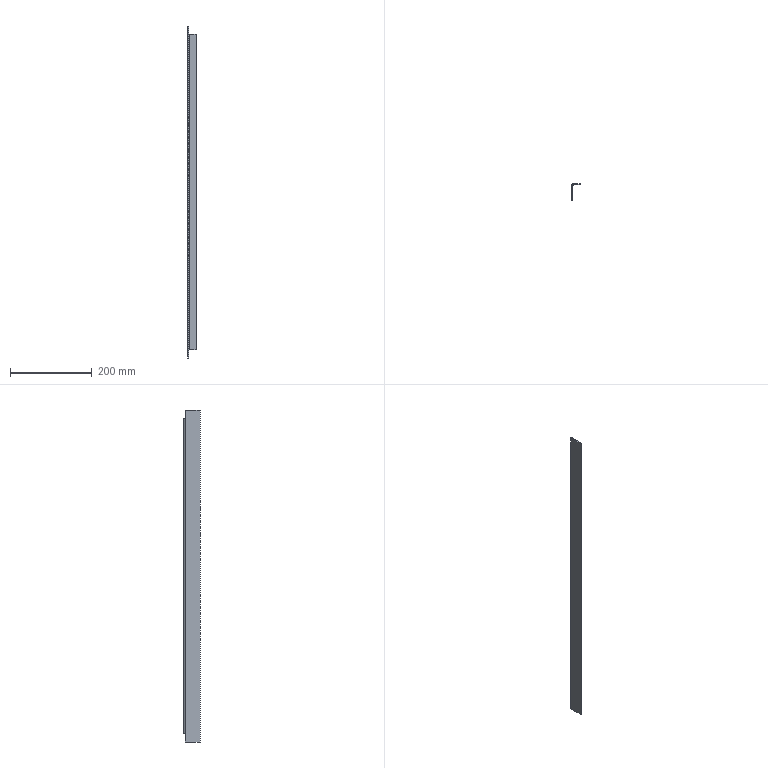Part | SolidWorks | features SMBaseFlange 2, FlatPattern 1, SheetMetal 1 | 1 solid | 16 faces | box 20 x 40 x 810 mm | volume 90217 mm3 | plane 14 | cylinder 2 | commonest cylinder face diameters 4 x1 8 x1
STEP:
#1=CARTESIAN_POINT('',(4.,40.,770.));
#2=VERTEX_POINT('',#1);
#3=CARTESIAN_POINT('',(4.,38.,770.));
#4=VERTEX_POINT('',#3);
#5=CARTESIAN_POINT('',(4.,40.,770.));
#6=DIRECTION('',(0.,-1.,0.));
#7=VECTOR('',#6,1000.);
#8=LINE('',#5,#7);
#9=EDGE_CURVE('',#2,#4,#8,.T.);
#10=ORIENTED_EDGE('',*,*,#9,.F.);
#11=CARTESIAN_POINT('',(0.,36.,770.));
#12=VERTEX_POINT('',#11);
#13=CARTESIAN_POINT('',(4.,36.,770.));
#14=DIRECTION('',(0.,0.,-1.));
#15=DIRECTION('',(1.,0.,0.));
#16=AXIS2_PLACEMENT_3D('',#13,#14,#15);
#17=CIRCLE('',#16,4.);
#18=EDGE_CURVE('',#12,#2,#17,.T.);
#19=ORIENTED_EDGE('',*,*,#18,.F.);
#20=CARTESIAN_POINT('',(2.,36.,770.));
#21=VERTEX_POINT('',#20);
#22=CARTESIAN_POINT('',(2.,36.,770.));
#23=DIRECTION('',(-1.,0.,0.));
#24=VECTOR('',#23,1000.);
#25=LINE('',#22,#24);
#26=EDGE_CURVE('',#21,#12,#25,.T.);
#27=ORIENTED_EDGE('',*,*,#26,.F.);
#28=CARTESIAN_POINT('',(4.,36.,770.));
#29=DIRECTION('',(0.,0.,-1.));
#30=DIRECTION('',(1.,0.,0.));
#31=AXIS2_PLACEMENT_3D('',#28,#29,#30);
#32=CIRCLE('',#31,2.);
#33=EDGE_CURVE('',#21,#4,#32,.T.);
#34=ORIENTED_EDGE('',*,*,#33,.T.);
#35=EDGE_LOOP('',(#10,#19,#27,#34));
#36=FACE_OUTER_BOUND('',#35,.T.);
#37=CARTESIAN_POINT('',(4.,40.,770.));
#38=DIRECTION('',(0.,0.,1.));
#39=DIRECTION('',(1.,0.,0.));
#40=AXIS2_PLACEMENT_3D('',#37,#38,#39);
#41=PLANE('',#40);
#42=ADVANCED_FACE('',(#36),#41,.T.);
#43=CARTESIAN_POINT('',(20.,40.,770.));
#44=VERTEX_POINT('',#43);
#45=CARTESIAN_POINT('',(0.,40.,770.));
#46=DIRECTION('',(1.,0.,0.));
#47=VECTOR('',#46,1000.);
#48=LINE('',#45,#47);
#49=EDGE_CURVE('',#2,#44,#48,.T.);
#50=ORIENTED_EDGE('',*,*,#49,.F.);
#51=ORIENTED_EDGE('',*,*,#9,.T.);
#52=CARTESIAN_POINT('',(20.,38.,770.));
#53=VERTEX_POINT('',#52);
#54=CARTESIAN_POINT('',(0.,38.,770.));
#55=DIRECTION('',(1.,0.,0.));
#56=VECTOR('',#55,1000.);
#57=LINE('',#54,#56);
#58=EDGE_CURVE('',#4,#53,#57,.T.);
#59=ORIENTED_EDGE('',*,*,#58,.T.);
#60=CARTESIAN_POINT('',(20.,40.,770.));
#61=DIRECTION('',(0.,-1.,0.));
#62=VECTOR('',#61,1000.);
#63=LINE('',#60,#62);
#64=EDGE_CURVE('',#44,#53,#63,.T.);
#65=ORIENTED_EDGE('',*,*,#64,.F.);
#66=EDGE_LOOP('',(#50,#51,#59,#65));
#67=FACE_OUTER_BOUND('',#66,.T.);
#68=CARTESIAN_POINT('',(2.,36.,770.));
#69=DIRECTION('',(0.,0.,1.));
#70=DIRECTION('',(1.,0.,0.));
#71=AXIS2_PLACEMENT_3D('',#68,#69,#70);
#72=PLANE('',#71);
#73=ADVANCED_FACE('',(#67),#72,.T.);
#74=CARTESIAN_POINT('',(0.,36.,0.));
#75=VERTEX_POINT('',#74);
#76=CARTESIAN_POINT('',(2.,36.,0.));
#77=VERTEX_POINT('',#76);
#78=CARTESIAN_POINT('',(0.,36.,0.));
#79=DIRECTION('',(1.,0.,0.));
#80=VECTOR('',#79,1000.);
#81=LINE('',#78,#80);
#82=EDGE_CURVE('',#75,#77,#81,.T.);
#83=ORIENTED_EDGE('',*,*,#82,.F.);
#84=CARTESIAN_POINT('',(4.,40.,0.));
#85=VERTEX_POINT('',#84);
#86=CARTESIAN_POINT('',(4.,36.,0.));
#87=DIRECTION('',(0.,0.,-1.));
#88=DIRECTION('',(1.,0.,0.));
#89=AXIS2_PLACEMENT_3D('',#86,#87,#88);
#90=CIRCLE('',#89,4.);
#91=EDGE_CURVE('',#75,#85,#90,.T.);
#92=ORIENTED_EDGE('',*,*,#91,.T.);
#93=CARTESIAN_POINT('',(4.,38.,0.));
#94=VERTEX_POINT('',#93);
#95=CARTESIAN_POINT('',(4.,38.,0.));
#96=DIRECTION('',(0.,1.,0.));
#97=VECTOR('',#96,1000.);
#98=LINE('',#95,#97);
#99=EDGE_CURVE('',#94,#85,#98,.T.);
#100=ORIENTED_EDGE('',*,*,#99,.F.);
#101=CARTESIAN_POINT('',(4.,36.,0.));
#102=DIRECTION('',(0.,0.,-1.));
#103=DIRECTION('',(1.,0.,0.));
#104=AXIS2_PLACEMENT_3D('',#101,#102,#103);
#105=CIRCLE('',#104,2.);
#106=EDGE_CURVE('',#77,#94,#105,.T.);
#107=ORIENTED_EDGE('',*,*,#106,.F.);
#108=EDGE_LOOP('',(#83,#92,#100,#107));
#109=FACE_OUTER_BOUND('',#108,.T.);
#110=CARTESIAN_POINT('',(0.,36.,0.));
#111=DIRECTION('',(0.,0.,-1.));
#112=DIRECTION('',(-1.,0.,0.));
#113=AXIS2_PLACEMENT_3D('',#110,#111,#112);
#114=PLANE('',#113);
#115=ADVANCED_FACE('',(#109),#114,.T.);
#116=CARTESIAN_POINT('',(20.,38.,0.));
#117=VERTEX_POINT('',#116);
#118=CARTESIAN_POINT('',(0.,38.,0.));
#119=DIRECTION('',(1.,0.,0.));
#120=VECTOR('',#119,1000.);
#121=LINE('',#118,#120);
#122=EDGE_CURVE('',#94,#117,#121,.T.);
#123=ORIENTED_EDGE('',*,*,#122,.T.);
#124=CARTESIAN_POINT('',(20.,38.,770.));
#125=DIRECTION('',(0.,0.,-1.));
#126=VECTOR('',#125,1000.);
#127=LINE('',#124,#126);
#128=EDGE_CURVE('',#53,#117,#127,.T.);
#129=ORIENTED_EDGE('',*,*,#128,.F.);
#130=ORIENTED_EDGE('',*,*,#58,.F.);
#131=CARTESIAN_POINT('',(4.,38.,770.));
#132=DIRECTION('',(0.,0.,-1.));
#133=VECTOR('',#132,1000.);
#134=LINE('',#131,#133);
#135=EDGE_CURVE('',#4,#94,#134,.T.);
#136=ORIENTED_EDGE('',*,*,#135,.T.);
#137=EDGE_LOOP('',(#123,#129,#130,#136));
#138=FACE_OUTER_BOUND('',#137,.T.);
#139=CARTESIAN_POINT('',(0.,38.,770.));
#140=DIRECTION('',(0.,1.,0.));
#141=DIRECTION('',(0.,0.,1.));
#142=AXIS2_PLACEMENT_3D('',#139,#140,#141);
#143=PLANE('',#142);
#144=ADVANCED_FACE('',(#138),#143,.F.);
#145=CARTESIAN_POINT('',(20.,40.,0.));
#146=VERTEX_POINT('',#145);
#147=CARTESIAN_POINT('',(20.,40.,0.));
#148=DIRECTION('',(0.,-1.,0.));
#149=VECTOR('',#148,1000.);
#150=LINE('',#147,#149);
#151=EDGE_CURVE('',#146,#117,#150,.T.);
#152=ORIENTED_EDGE('',*,*,#151,.F.);
#153=CARTESIAN_POINT('',(20.,40.,770.));
#154=DIRECTION('',(0.,0.,-1.));
#155=VECTOR('',#154,1000.);
#156=LINE('',#153,#155);
#157=EDGE_CURVE('',#44,#146,#156,.T.);
#158=ORIENTED_EDGE('',*,*,#157,.F.);
#159=ORIENTED_EDGE('',*,*,#64,.T.);
#160=ORIENTED_EDGE('',*,*,#128,.T.);
#161=EDGE_LOOP('',(#152,#158,#159,#160));
#162=FACE_OUTER_BOUND('',#161,.T.);
#163=CARTESIAN_POINT('',(20.,40.,770.));
#164=DIRECTION('',(1.,0.,0.));
#165=DIRECTION('',(0.,0.,-1.));
#166=AXIS2_PLACEMENT_3D('',#163,#164,#165);
#167=PLANE('',#166);
#168=ADVANCED_FACE('',(#162),#167,.T.);
#169=CARTESIAN_POINT('',(0.,40.,0.));
#170=DIRECTION('',(1.,0.,0.));
#171=VECTOR('',#170,1000.);
#172=LINE('',#169,#171);
#173=EDGE_CURVE('',#85,#146,#172,.T.);
#174=ORIENTED_EDGE('',*,*,#173,.F.);
#175=CARTESIAN_POINT('',(4.,40.,770.));
#176=DIRECTION('',(0.,0.,-1.));
#177=VECTOR('',#176,1000.);
#178=LINE('',#175,#177);
#179=EDGE_CURVE('',#2,#85,#178,.T.);
#180=ORIENTED_EDGE('',*,*,#179,.F.);
#181=ORIENTED_EDGE('',*,*,#49,.T.);
#182=ORIENTED_EDGE('',*,*,#157,.T.);
#183=EDGE_LOOP('',(#174,#180,#181,#182));
#184=FACE_OUTER_BOUND('',#183,.T.);
#185=CARTESIAN_POINT('',(0.,40.,770.));
#186=DIRECTION('',(0.,1.,0.));
#187=DIRECTION('',(0.,0.,1.));
#188=AXIS2_PLACEMENT_3D('',#185,#186,#187);
#189=PLANE('',#188);
#190=ADVANCED_FACE('',(#184),#189,.T.);
#191=ORIENTED_EDGE('',*,*,#91,.F.);
#192=CARTESIAN_POINT('',(0.,36.,770.));
#193=DIRECTION('',(0.,0.,-1.));
#194=VECTOR('',#193,1000.);
#195=LINE('',#192,#194);
#196=EDGE_CURVE('',#12,#75,#195,.T.);
#197=ORIENTED_EDGE('',*,*,#196,.F.);
#198=ORIENTED_EDGE('',*,*,#18,.T.);
#199=ORIENTED_EDGE('',*,*,#179,.T.);
#200=EDGE_LOOP('',(#191,#197,#198,#199));
#201=FACE_OUTER_BOUND('',#200,.T.);
#202=CARTESIAN_POINT('',(4.,36.,770.));
#203=DIRECTION('',(0.,0.,-1.));
#204=DIRECTION('',(-1.,0.,0.));
#205=AXIS2_PLACEMENT_3D('',#202,#203,#204);
#206=CYLINDRICAL_SURFACE('',#205,4.);
#207=ADVANCED_FACE('',(#201),#206,.T.);
#208=ORIENTED_EDGE('',*,*,#196,.T.);
#209=CARTESIAN_POINT('',(0.,36.,-20.));
#210=VERTEX_POINT('',#209);
#211=CARTESIAN_POINT('',(0.,36.,0.));
#212=DIRECTION('',(0.,0.,1.));
#213=VECTOR('',#212,1000.);
#214=LINE('',#211,#213);
#215=EDGE_CURVE('',#210,#75,#214,.T.);
#216=ORIENTED_EDGE('',*,*,#215,.F.);
#217=CARTESIAN_POINT('',(0.,0.,-20.));
#218=VERTEX_POINT('',#217);
#219=CARTESIAN_POINT('',(0.,0.,-20.));
#220=DIRECTION('',(0.,1.,0.));
#221=VECTOR('',#220,1000.);
#222=LINE('',#219,#221);
#223=EDGE_CURVE('',#218,#210,#222,.T.);
#224=ORIENTED_EDGE('',*,*,#223,.F.);
#225=CARTESIAN_POINT('',(0.,0.,790.));
#226=VERTEX_POINT('',#225);
#227=CARTESIAN_POINT('',(0.,0.,770.));
#228=DIRECTION('',(0.,0.,-1.));
#229=VECTOR('',#228,1000.);
#230=LINE('',#227,#229);
#231=EDGE_CURVE('',#226,#218,#230,.T.);
#232=ORIENTED_EDGE('',*,*,#231,.F.);
#233=CARTESIAN_POINT('',(0.,36.,790.));
#234=VERTEX_POINT('',#233);
#235=CARTESIAN_POINT('',(0.,0.,790.));
#236=DIRECTION('',(0.,-1.,0.));
#237=VECTOR('',#236,1000.);
#238=LINE('',#235,#237);
#239=EDGE_CURVE('',#234,#226,#238,.T.);
#240=ORIENTED_EDGE('',*,*,#239,.F.);
#241=CARTESIAN_POINT('',(0.,36.,770.));
#242=DIRECTION('',(0.,0.,1.));
#243=VECTOR('',#242,1000.);
#244=LINE('',#241,#243);
#245=EDGE_CURVE('',#12,#234,#244,.T.);
#246=ORIENTED_EDGE('',*,*,#245,.F.);
#247=EDGE_LOOP('',(#208,#216,#224,#232,#240,#246));
#248=FACE_OUTER_BOUND('',#247,.T.);
#249=CARTESIAN_POINT('',(0.,0.,770.));
#250=DIRECTION('',(-1.,0.,0.));
#251=DIRECTION('',(0.,0.,1.));
#252=AXIS2_PLACEMENT_3D('',#249,#250,#251);
#253=PLANE('',#252);
#254=ADVANCED_FACE('',(#248),#253,.T.);
#255=ORIENTED_EDGE('',*,*,#231,.T.);
#256=CARTESIAN_POINT('',(2.,0.,-20.));
#257=VERTEX_POINT('',#256);
#258=CARTESIAN_POINT('',(0.,0.,-20.));
#259=DIRECTION('',(1.,0.,0.));
#260=VECTOR('',#259,1000.);
#261=LINE('',#258,#260);
#262=EDGE_CURVE('',#218,#257,#261,.T.);
#263=ORIENTED_EDGE('',*,*,#262,.T.);
#264=CARTESIAN_POINT('',(2.,0.,790.));
#265=VERTEX_POINT('',#264);
#266=CARTESIAN_POINT('',(2.,0.,770.));
#267=DIRECTION('',(0.,0.,-1.));
#268=VECTOR('',#267,1000.);
#269=LINE('',#266,#268);
#270=EDGE_CURVE('',#265,#257,#269,.T.);
#271=ORIENTED_EDGE('',*,*,#270,.F.);
#272=CARTESIAN_POINT('',(0.,0.,790.));
#273=DIRECTION('',(1.,0.,0.));
#274=VECTOR('',#273,1000.);
#275=LINE('',#272,#274);
#276=EDGE_CURVE('',#226,#265,#275,.T.);
#277=ORIENTED_EDGE('',*,*,#276,.F.);
#278=EDGE_LOOP('',(#255,#263,#271,#277));
#279=FACE_OUTER_BOUND('',#278,.T.);
#280=CARTESIAN_POINT('',(2.,0.,770.));
#281=DIRECTION('',(0.,-1.,0.));
#282=DIRECTION('',(0.,0.,-1.));
#283=AXIS2_PLACEMENT_3D('',#280,#281,#282);
#284=PLANE('',#283);
#285=ADVANCED_FACE('',(#279),#284,.T.);
#286=ORIENTED_EDGE('',*,*,#270,.T.);
#287=CARTESIAN_POINT('',(2.,36.,-20.));
#288=VERTEX_POINT('',#287);
#289=CARTESIAN_POINT('',(2.,0.,-20.));
#290=DIRECTION('',(0.,1.,0.));
#291=VECTOR('',#290,1000.);
#292=LINE('',#289,#291);
#293=EDGE_CURVE('',#257,#288,#292,.T.);
#294=ORIENTED_EDGE('',*,*,#293,.T.);
#295=CARTESIAN_POINT('',(2.,36.,0.));
#296=DIRECTION('',(0.,0.,1.));
#297=VECTOR('',#296,1000.);
#298=LINE('',#295,#297);
#299=EDGE_CURVE('',#288,#77,#298,.T.);
#300=ORIENTED_EDGE('',*,*,#299,.T.);
#301=CARTESIAN_POINT('',(2.,36.,770.));
#302=DIRECTION('',(0.,0.,-1.));
#303=VECTOR('',#302,1000.);
#304=LINE('',#301,#303);
#305=EDGE_CURVE('',#21,#77,#304,.T.);
#306=ORIENTED_EDGE('',*,*,#305,.F.);
#307=CARTESIAN_POINT('',(2.,36.,790.));
#308=VERTEX_POINT('',#307);
#309=CARTESIAN_POINT('',(2.,36.,770.));
#310=DIRECTION('',(0.,0.,1.));
#311=VECTOR('',#310,1000.);
#312=LINE('',#309,#311);
#313=EDGE_CURVE('',#21,#308,#312,.T.);
#314=ORIENTED_EDGE('',*,*,#313,.T.);
#315=CARTESIAN_POINT('',(2.,0.,790.));
#316=DIRECTION('',(0.,-1.,0.));
#317=VECTOR('',#316,1000.);
#318=LINE('',#315,#317);
#319=EDGE_CURVE('',#308,#265,#318,.T.);
#320=ORIENTED_EDGE('',*,*,#319,.T.);
#321=EDGE_LOOP('',(#286,#294,#300,#306,#314,#320));
#322=FACE_OUTER_BOUND('',#321,.T.);
#323=CARTESIAN_POINT('',(2.,0.,770.));
#324=DIRECTION('',(-1.,0.,0.));
#325=DIRECTION('',(0.,0.,1.));
#326=AXIS2_PLACEMENT_3D('',#323,#324,#325);
#327=PLANE('',#326);
#328=ADVANCED_FACE('',(#322),#327,.F.);
#329=ORIENTED_EDGE('',*,*,#106,.T.);
#330=ORIENTED_EDGE('',*,*,#135,.F.);
#331=ORIENTED_EDGE('',*,*,#33,.F.);
#332=ORIENTED_EDGE('',*,*,#305,.T.);
#333=EDGE_LOOP('',(#329,#330,#331,#332));
#334=FACE_OUTER_BOUND('',#333,.T.);
#335=CARTESIAN_POINT('',(4.,36.,770.));
#336=DIRECTION('',(0.,0.,-1.));
#337=DIRECTION('',(-1.,0.,0.));
#338=AXIS2_PLACEMENT_3D('',#335,#336,#337);
#339=CYLINDRICAL_SURFACE('',#338,2.);
#340=ADVANCED_FACE('',(#334),#339,.F.);
#341=ORIENTED_EDGE('',*,*,#122,.F.);
#342=ORIENTED_EDGE('',*,*,#99,.T.);
#343=ORIENTED_EDGE('',*,*,#173,.T.);
#344=ORIENTED_EDGE('',*,*,#151,.T.);
#345=EDGE_LOOP('',(#341,#342,#343,#344));
#346=FACE_OUTER_BOUND('',#345,.T.);
#347=CARTESIAN_POINT('',(4.,36.,0.));
#348=DIRECTION('',(0.,0.,1.));
#349=DIRECTION('',(1.,0.,0.));
#350=AXIS2_PLACEMENT_3D('',#347,#348,#349);
#351=PLANE('',#350);
#352=ADVANCED_FACE('',(#346),#351,.F.);
#353=ORIENTED_EDGE('',*,*,#319,.F.);
#354=CARTESIAN_POINT('',(0.,36.,790.));
#355=DIRECTION('',(1.,0.,0.));
#356=VECTOR('',#355,1000.);
#357=LINE('',#354,#356);
#358=EDGE_CURVE('',#234,#308,#357,.T.);
#359=ORIENTED_EDGE('',*,*,#358,.F.);
#360=ORIENTED_EDGE('',*,*,#239,.T.);
#361=ORIENTED_EDGE('',*,*,#276,.T.);
#362=EDGE_LOOP('',(#353,#359,#360,#361));
#363=FACE_OUTER_BOUND('',#362,.T.);
#364=CARTESIAN_POINT('',(0.,0.,790.));
#365=DIRECTION('',(0.,0.,1.));
#366=DIRECTION('',(1.,0.,0.));
#367=AXIS2_PLACEMENT_3D('',#364,#365,#366);
#368=PLANE('',#367);
#369=ADVANCED_FACE('',(#363),#368,.T.);
#370=ORIENTED_EDGE('',*,*,#313,.F.);
#371=ORIENTED_EDGE('',*,*,#26,.T.);
#372=ORIENTED_EDGE('',*,*,#245,.T.);
#373=ORIENTED_EDGE('',*,*,#358,.T.);
#374=EDGE_LOOP('',(#370,#371,#372,#373));
#375=FACE_OUTER_BOUND('',#374,.T.);
#376=CARTESIAN_POINT('',(0.,36.,770.));
#377=DIRECTION('',(0.,1.,0.));
#378=DIRECTION('',(0.,0.,1.));
#379=AXIS2_PLACEMENT_3D('',#376,#377,#378);
#380=PLANE('',#379);
#381=ADVANCED_FACE('',(#375),#380,.T.);
#382=ORIENTED_EDGE('',*,*,#299,.F.);
#383=CARTESIAN_POINT('',(0.,36.,-20.));
#384=DIRECTION('',(1.,0.,0.));
#385=VECTOR('',#384,1000.);
#386=LINE('',#383,#385);
#387=EDGE_CURVE('',#210,#288,#386,.T.);
#388=ORIENTED_EDGE('',*,*,#387,.F.);
#389=ORIENTED_EDGE('',*,*,#215,.T.);
#390=ORIENTED_EDGE('',*,*,#82,.T.);
#391=EDGE_LOOP('',(#382,#388,#389,#390));
#392=FACE_OUTER_BOUND('',#391,.T.);
#393=CARTESIAN_POINT('',(0.,36.,0.));
#394=DIRECTION('',(0.,1.,0.));
#395=DIRECTION('',(0.,0.,1.));
#396=AXIS2_PLACEMENT_3D('',#393,#394,#395);
#397=PLANE('',#396);
#398=ADVANCED_FACE('',(#392),#397,.T.);
#399=ORIENTED_EDGE('',*,*,#293,.F.);
#400=ORIENTED_EDGE('',*,*,#262,.F.);
#401=ORIENTED_EDGE('',*,*,#223,.T.);
#402=ORIENTED_EDGE('',*,*,#387,.T.);
#403=EDGE_LOOP('',(#399,#400,#401,#402));
#404=FACE_OUTER_BOUND('',#403,.T.);
#405=CARTESIAN_POINT('',(0.,0.,-20.));
#406=DIRECTION('',(0.,0.,-1.));
#407=DIRECTION('',(-1.,0.,0.));
#408=AXIS2_PLACEMENT_3D('',#405,#406,#407);
#409=PLANE('',#408);
#410=ADVANCED_FACE('',(#404),#409,.T.);
#411=CLOSED_SHELL('',(#42,#73,#115,#144,#168,#190,#207,#254,#285,#328,#340,#352,#369,#381,#398,#410));
#412=MANIFOLD_SOLID_BREP('',#411);
#413=CARTESIAN_POINT('',(0.,0.,0.));
#414=DIRECTION('',(0.,0.,1.));
#415=DIRECTION('',(1.,0.,0.));
#416=AXIS2_PLACEMENT_3D('',#413,#414,#415);
#417=(LENGTH_UNIT()NAMED_UNIT(*)SI_UNIT(.MILLI.,.METRE.));
#418=UNCERTAINTY_MEASURE_WITH_UNIT(LENGTH_MEASURE(0.00001),#417,'','');
#419=(NAMED_UNIT(*)PLANE_ANGLE_UNIT()SI_UNIT($,.RADIAN.));
#420=(NAMED_UNIT(*)SI_UNIT($,.STERADIAN.)SOLID_ANGLE_UNIT());
#421=(GEOMETRIC_REPRESENTATION_CONTEXT(3)GLOBAL_UNCERTAINTY_ASSIGNED_CONTEXT((#418))GLOBAL_UNIT_ASSIGNED_CONTEXT((#417,#419,#420))REPRESENTATION_CONTEXT('',''));
#422=ADVANCED_BREP_SHAPE_REPRESENTATION('',(#412,#416),#421);